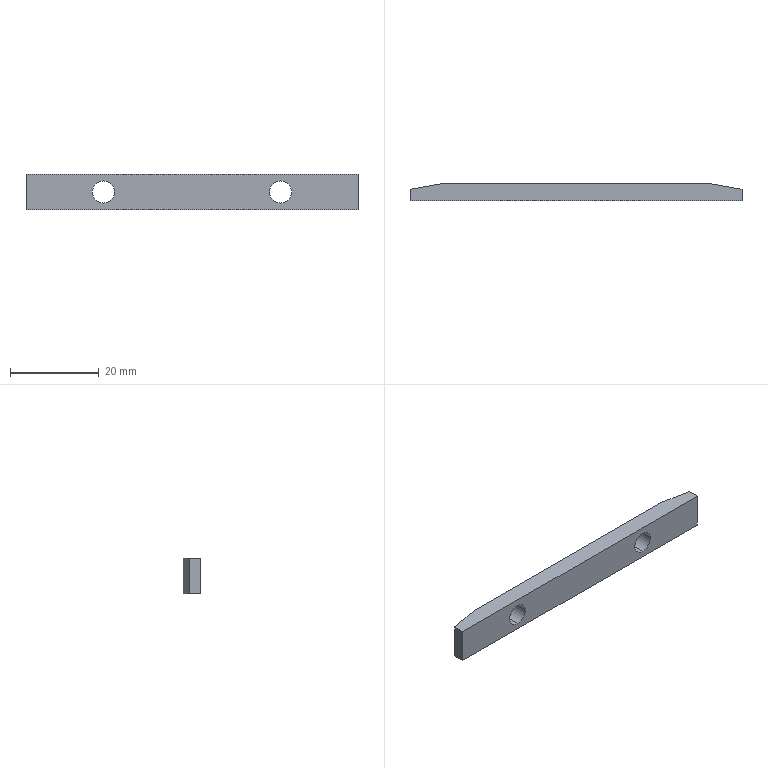Part | SolidWorks | features Chamfer 5, ICE 4, HoleWzd 2, Extrusion 1, Fillet 1 | 1 solid | 12 faces | box 75 x 4 x 8 mm | volume 2157 mm3 | plane 8 | cylinder 4 | commonest cylinder face diameters 5 x4
STEP:
#1=CARTESIAN_POINT('',(20.,45.,-2.5));
#2=VERTEX_POINT('',#1);
#3=CARTESIAN_POINT('',(20.,45.,2.5));
#4=VERTEX_POINT('',#3);
#5=CARTESIAN_POINT('',(20.,45.,0.));
#6=DIRECTION('',(0.,1.,0.));
#7=DIRECTION('',(0.,0.,1.));
#8=AXIS2_PLACEMENT_3D('',#5,#6,#7);
#9=CIRCLE('',#8,2.5);
#10=EDGE_CURVE('',#2,#4,#9,.T.);
#11=ORIENTED_EDGE('',*,*,#10,.F.);
#12=CARTESIAN_POINT('',(20.,49.,-2.5));
#13=VERTEX_POINT('',#12);
#14=CARTESIAN_POINT('',(20.,32.5,-2.5));
#15=DIRECTION('',(0.,1.,0.));
#16=VECTOR('',#15,1000.);
#17=LINE('',#14,#16);
#18=EDGE_CURVE('',#2,#13,#17,.T.);
#19=ORIENTED_EDGE('',*,*,#18,.T.);
#20=CARTESIAN_POINT('',(20.,49.,2.5));
#21=VERTEX_POINT('',#20);
#22=CARTESIAN_POINT('',(20.,49.,0.));
#23=DIRECTION('',(0.,1.,0.));
#24=DIRECTION('',(0.,0.,1.));
#25=AXIS2_PLACEMENT_3D('',#22,#23,#24);
#26=CIRCLE('',#25,2.5);
#27=EDGE_CURVE('',#13,#21,#26,.T.);
#28=ORIENTED_EDGE('',*,*,#27,.T.);
#29=CARTESIAN_POINT('',(20.,32.5,2.5));
#30=DIRECTION('',(0.,1.,0.));
#31=VECTOR('',#30,1000.);
#32=LINE('',#29,#31);
#33=EDGE_CURVE('',#4,#21,#32,.T.);
#34=ORIENTED_EDGE('',*,*,#33,.F.);
#35=EDGE_LOOP('',(#11,#19,#28,#34));
#36=FACE_OUTER_BOUND('',#35,.T.);
#37=CARTESIAN_POINT('',(20.,32.5,0.));
#38=DIRECTION('',(0.,1.,0.));
#39=DIRECTION('',(0.,0.,1.));
#40=AXIS2_PLACEMENT_3D('',#37,#38,#39);
#41=CYLINDRICAL_SURFACE('',#40,2.5);
#42=ADVANCED_FACE('',(#36),#41,.F.);
#43=CARTESIAN_POINT('',(-20.,45.,-2.5));
#44=VERTEX_POINT('',#43);
#45=CARTESIAN_POINT('',(-20.,45.,2.5));
#46=VERTEX_POINT('',#45);
#47=CARTESIAN_POINT('',(-20.,45.,0.));
#48=DIRECTION('',(0.,1.,0.));
#49=DIRECTION('',(0.,0.,1.));
#50=AXIS2_PLACEMENT_3D('',#47,#48,#49);
#51=CIRCLE('',#50,2.5);
#52=EDGE_CURVE('',#44,#46,#51,.T.);
#53=ORIENTED_EDGE('',*,*,#52,.F.);
#54=CARTESIAN_POINT('',(-20.,49.,-2.5));
#55=VERTEX_POINT('',#54);
#56=CARTESIAN_POINT('',(-20.,32.5,-2.5));
#57=DIRECTION('',(0.,1.,0.));
#58=VECTOR('',#57,1000.);
#59=LINE('',#56,#58);
#60=EDGE_CURVE('',#44,#55,#59,.T.);
#61=ORIENTED_EDGE('',*,*,#60,.T.);
#62=CARTESIAN_POINT('',(-20.,49.,2.5));
#63=VERTEX_POINT('',#62);
#64=CARTESIAN_POINT('',(-20.,49.,0.));
#65=DIRECTION('',(0.,1.,0.));
#66=DIRECTION('',(0.,0.,1.));
#67=AXIS2_PLACEMENT_3D('',#64,#65,#66);
#68=CIRCLE('',#67,2.5);
#69=EDGE_CURVE('',#55,#63,#68,.T.);
#70=ORIENTED_EDGE('',*,*,#69,.T.);
#71=CARTESIAN_POINT('',(-20.,32.5,2.5));
#72=DIRECTION('',(0.,1.,0.));
#73=VECTOR('',#72,1000.);
#74=LINE('',#71,#73);
#75=EDGE_CURVE('',#46,#63,#74,.T.);
#76=ORIENTED_EDGE('',*,*,#75,.F.);
#77=EDGE_LOOP('',(#53,#61,#70,#76));
#78=FACE_OUTER_BOUND('',#77,.T.);
#79=CARTESIAN_POINT('',(-20.,32.5,0.));
#80=DIRECTION('',(0.,1.,0.));
#81=DIRECTION('',(0.,0.,1.));
#82=AXIS2_PLACEMENT_3D('',#79,#80,#81);
#83=CYLINDRICAL_SURFACE('',#82,2.5);
#84=ADVANCED_FACE('',(#78),#83,.F.);
#85=CARTESIAN_POINT('',(37.5,45.,4.));
#86=VERTEX_POINT('',#85);
#87=CARTESIAN_POINT('',(-37.5,45.,4.));
#88=VERTEX_POINT('',#87);
#89=CARTESIAN_POINT('',(-71.258,45.,4.));
#90=DIRECTION('',(-1.,0.,0.));
#91=VECTOR('',#90,1000.);
#92=LINE('',#89,#91);
#93=EDGE_CURVE('',#86,#88,#92,.T.);
#94=ORIENTED_EDGE('',*,*,#93,.F.);
#95=CARTESIAN_POINT('',(37.5,47.6,4.));
#96=VERTEX_POINT('',#95);
#97=CARTESIAN_POINT('',(37.5,49.,4.));
#98=DIRECTION('',(0.,1.,0.));
#99=VECTOR('',#98,1000.);
#100=LINE('',#97,#99);
#101=EDGE_CURVE('',#86,#96,#100,.T.);
#102=ORIENTED_EDGE('',*,*,#101,.T.);
#103=CARTESIAN_POINT('',(29.8,49.,4.));
#104=VERTEX_POINT('',#103);
#105=CARTESIAN_POINT('',(9.578,52.677,4.));
#106=DIRECTION('',(-0.9839,0.1789,0.));
#107=VECTOR('',#106,1000.);
#108=LINE('',#105,#107);
#109=EDGE_CURVE('',#96,#104,#108,.T.);
#110=ORIENTED_EDGE('',*,*,#109,.T.);
#111=CARTESIAN_POINT('',(-29.8,49.,4.));
#112=VERTEX_POINT('',#111);
#113=CARTESIAN_POINT('',(-37.5,49.,4.));
#114=DIRECTION('',(-1.,0.,0.));
#115=VECTOR('',#114,1000.);
#116=LINE('',#113,#115);
#117=EDGE_CURVE('',#104,#112,#116,.T.);
#118=ORIENTED_EDGE('',*,*,#117,.T.);
#119=CARTESIAN_POINT('',(-37.5,47.6,4.));
#120=VERTEX_POINT('',#119);
#121=CARTESIAN_POINT('',(-9.578,52.677,4.));
#122=DIRECTION('',(-0.9839,-0.1789,0.));
#123=VECTOR('',#122,1000.);
#124=LINE('',#121,#123);
#125=EDGE_CURVE('',#112,#120,#124,.T.);
#126=ORIENTED_EDGE('',*,*,#125,.T.);
#127=CARTESIAN_POINT('',(-37.5,49.,4.));
#128=DIRECTION('',(0.,-1.,0.));
#129=VECTOR('',#128,1000.);
#130=LINE('',#127,#129);
#131=EDGE_CURVE('',#120,#88,#130,.T.);
#132=ORIENTED_EDGE('',*,*,#131,.T.);
#133=EDGE_LOOP('',(#94,#102,#110,#118,#126,#132));
#134=FACE_OUTER_BOUND('',#133,.T.);
#135=CARTESIAN_POINT('',(0.,0.,4.));
#136=DIRECTION('',(0.,0.,1.));
#137=DIRECTION('',(1.,0.,0.));
#138=AXIS2_PLACEMENT_3D('',#135,#136,#137);
#139=PLANE('',#138);
#140=ADVANCED_FACE('',(#134),#139,.T.);
#141=CARTESIAN_POINT('',(37.5,45.,-4.));
#142=VERTEX_POINT('',#141);
#143=CARTESIAN_POINT('',(37.5,47.6,-4.));
#144=VERTEX_POINT('',#143);
#145=CARTESIAN_POINT('',(37.5,49.,-4.));
#146=DIRECTION('',(0.,1.,0.));
#147=VECTOR('',#146,1000.);
#148=LINE('',#145,#147);
#149=EDGE_CURVE('',#142,#144,#148,.T.);
#150=ORIENTED_EDGE('',*,*,#149,.F.);
#151=CARTESIAN_POINT('',(-37.5,45.,-4.));
#152=VERTEX_POINT('',#151);
#153=CARTESIAN_POINT('',(0.,45.,-4.));
#154=DIRECTION('',(-1.,0.,0.));
#155=VECTOR('',#154,1000.);
#156=LINE('',#153,#155);
#157=EDGE_CURVE('',#142,#152,#156,.T.);
#158=ORIENTED_EDGE('',*,*,#157,.T.);
#159=CARTESIAN_POINT('',(-37.5,47.6,-4.));
#160=VERTEX_POINT('',#159);
#161=CARTESIAN_POINT('',(-37.5,49.,-4.));
#162=DIRECTION('',(0.,-1.,0.));
#163=VECTOR('',#162,1000.);
#164=LINE('',#161,#163);
#165=EDGE_CURVE('',#160,#152,#164,.T.);
#166=ORIENTED_EDGE('',*,*,#165,.F.);
#167=CARTESIAN_POINT('',(-29.8,49.,-4.));
#168=VERTEX_POINT('',#167);
#169=CARTESIAN_POINT('',(-37.5,47.6,-4.));
#170=DIRECTION('',(0.9839,0.1789,0.));
#171=VECTOR('',#170,1000.);
#172=LINE('',#169,#171);
#173=EDGE_CURVE('',#160,#168,#172,.T.);
#174=ORIENTED_EDGE('',*,*,#173,.T.);
#175=CARTESIAN_POINT('',(29.8,49.,-4.));
#176=VERTEX_POINT('',#175);
#177=CARTESIAN_POINT('',(-37.5,49.,-4.));
#178=DIRECTION('',(-1.,0.,0.));
#179=VECTOR('',#178,1000.);
#180=LINE('',#177,#179);
#181=EDGE_CURVE('',#176,#168,#180,.T.);
#182=ORIENTED_EDGE('',*,*,#181,.F.);
#183=CARTESIAN_POINT('',(29.8,49.,-4.));
#184=DIRECTION('',(0.9839,-0.1789,0.));
#185=VECTOR('',#184,1000.);
#186=LINE('',#183,#185);
#187=EDGE_CURVE('',#176,#144,#186,.T.);
#188=ORIENTED_EDGE('',*,*,#187,.T.);
#189=EDGE_LOOP('',(#150,#158,#166,#174,#182,#188));
#190=FACE_OUTER_BOUND('',#189,.T.);
#191=CARTESIAN_POINT('',(0.,0.,-4.));
#192=DIRECTION('',(0.,0.,1.));
#193=DIRECTION('',(1.,0.,0.));
#194=AXIS2_PLACEMENT_3D('',#191,#192,#193);
#195=PLANE('',#194);
#196=ADVANCED_FACE('',(#190),#195,.F.);
#197=ORIENTED_EDGE('',*,*,#101,.F.);
#198=CARTESIAN_POINT('',(37.5,45.,4.));
#199=DIRECTION('',(0.,0.,-1.));
#200=VECTOR('',#199,1000.);
#201=LINE('',#198,#200);
#202=EDGE_CURVE('',#86,#142,#201,.T.);
#203=ORIENTED_EDGE('',*,*,#202,.T.);
#204=ORIENTED_EDGE('',*,*,#149,.T.);
#205=CARTESIAN_POINT('',(37.5,47.6,4.));
#206=DIRECTION('',(0.,0.,1.));
#207=VECTOR('',#206,1000.);
#208=LINE('',#205,#207);
#209=EDGE_CURVE('',#144,#96,#208,.T.);
#210=ORIENTED_EDGE('',*,*,#209,.T.);
#211=EDGE_LOOP('',(#197,#203,#204,#210));
#212=FACE_OUTER_BOUND('',#211,.T.);
#213=CARTESIAN_POINT('',(37.5,49.,4.));
#214=DIRECTION('',(-1.,0.,0.));
#215=DIRECTION('',(0.,0.,1.));
#216=AXIS2_PLACEMENT_3D('',#213,#214,#215);
#217=PLANE('',#216);
#218=ADVANCED_FACE('',(#212),#217,.F.);
#219=CARTESIAN_POINT('',(20.,49.,0.));
#220=DIRECTION('',(0.,1.,0.));
#221=DIRECTION('',(0.,0.,1.));
#222=AXIS2_PLACEMENT_3D('',#219,#220,#221);
#223=CIRCLE('',#222,2.5);
#224=EDGE_CURVE('',#21,#13,#223,.T.);
#225=ORIENTED_EDGE('',*,*,#224,.F.);
#226=ORIENTED_EDGE('',*,*,#27,.F.);
#227=EDGE_LOOP('',(#225,#226));
#228=FACE_BOUND('',#227,.T.);
#229=CARTESIAN_POINT('',(-20.,49.,0.));
#230=DIRECTION('',(0.,1.,0.));
#231=DIRECTION('',(0.,0.,1.));
#232=AXIS2_PLACEMENT_3D('',#229,#230,#231);
#233=CIRCLE('',#232,2.5);
#234=EDGE_CURVE('',#63,#55,#233,.T.);
#235=ORIENTED_EDGE('',*,*,#234,.F.);
#236=ORIENTED_EDGE('',*,*,#69,.F.);
#237=EDGE_LOOP('',(#235,#236));
#238=FACE_BOUND('',#237,.T.);
#239=ORIENTED_EDGE('',*,*,#117,.F.);
#240=CARTESIAN_POINT('',(29.8,49.,4.));
#241=DIRECTION('',(0.,0.,-1.));
#242=VECTOR('',#241,1000.);
#243=LINE('',#240,#242);
#244=EDGE_CURVE('',#104,#176,#243,.T.);
#245=ORIENTED_EDGE('',*,*,#244,.T.);
#246=ORIENTED_EDGE('',*,*,#181,.T.);
#247=CARTESIAN_POINT('',(-29.8,49.,4.));
#248=DIRECTION('',(0.,0.,1.));
#249=VECTOR('',#248,1000.);
#250=LINE('',#247,#249);
#251=EDGE_CURVE('',#168,#112,#250,.T.);
#252=ORIENTED_EDGE('',*,*,#251,.T.);
#253=EDGE_LOOP('',(#239,#245,#246,#252));
#254=FACE_OUTER_BOUND('',#253,.T.);
#255=CARTESIAN_POINT('',(-37.5,49.,4.));
#256=DIRECTION('',(0.,-1.,0.));
#257=DIRECTION('',(0.,0.,-1.));
#258=AXIS2_PLACEMENT_3D('',#255,#256,#257);
#259=PLANE('',#258);
#260=ADVANCED_FACE('',(#228,#238,#254),#259,.F.);
#261=ORIENTED_EDGE('',*,*,#165,.T.);
#262=CARTESIAN_POINT('',(-37.5,45.,4.));
#263=DIRECTION('',(0.,0.,1.));
#264=VECTOR('',#263,1000.);
#265=LINE('',#262,#264);
#266=EDGE_CURVE('',#152,#88,#265,.T.);
#267=ORIENTED_EDGE('',*,*,#266,.T.);
#268=ORIENTED_EDGE('',*,*,#131,.F.);
#269=CARTESIAN_POINT('',(-37.5,47.6,4.));
#270=DIRECTION('',(0.,0.,-1.));
#271=VECTOR('',#270,1000.);
#272=LINE('',#269,#271);
#273=EDGE_CURVE('',#120,#160,#272,.T.);
#274=ORIENTED_EDGE('',*,*,#273,.T.);
#275=EDGE_LOOP('',(#261,#267,#268,#274));
#276=FACE_OUTER_BOUND('',#275,.T.);
#277=CARTESIAN_POINT('',(-37.5,49.,4.));
#278=DIRECTION('',(1.,0.,0.));
#279=DIRECTION('',(0.,1.,0.));
#280=AXIS2_PLACEMENT_3D('',#277,#278,#279);
#281=PLANE('',#280);
#282=ADVANCED_FACE('',(#276),#281,.F.);
#283=ORIENTED_EDGE('',*,*,#125,.F.);
#284=ORIENTED_EDGE('',*,*,#251,.F.);
#285=ORIENTED_EDGE('',*,*,#173,.F.);
#286=ORIENTED_EDGE('',*,*,#273,.F.);
#287=EDGE_LOOP('',(#283,#284,#285,#286));
#288=FACE_OUTER_BOUND('',#287,.T.);
#289=CARTESIAN_POINT('',(-37.5,47.6,4.));
#290=DIRECTION('',(0.1789,-0.9839,0.));
#291=DIRECTION('',(0.,0.,-1.));
#292=AXIS2_PLACEMENT_3D('',#289,#290,#291);
#293=PLANE('',#292);
#294=ADVANCED_FACE('',(#288),#293,.F.);
#295=ORIENTED_EDGE('',*,*,#109,.F.);
#296=ORIENTED_EDGE('',*,*,#209,.F.);
#297=ORIENTED_EDGE('',*,*,#187,.F.);
#298=ORIENTED_EDGE('',*,*,#244,.F.);
#299=EDGE_LOOP('',(#295,#296,#297,#298));
#300=FACE_OUTER_BOUND('',#299,.T.);
#301=CARTESIAN_POINT('',(29.8,49.,4.));
#302=DIRECTION('',(-0.1789,-0.9839,0.));
#303=DIRECTION('',(0.,0.,-1.));
#304=AXIS2_PLACEMENT_3D('',#301,#302,#303);
#305=PLANE('',#304);
#306=ADVANCED_FACE('',(#300),#305,.F.);
#307=CARTESIAN_POINT('',(20.,45.,0.));
#308=DIRECTION('',(0.,1.,0.));
#309=DIRECTION('',(0.,0.,1.));
#310=AXIS2_PLACEMENT_3D('',#307,#308,#309);
#311=CIRCLE('',#310,2.5);
#312=EDGE_CURVE('',#4,#2,#311,.T.);
#313=ORIENTED_EDGE('',*,*,#312,.T.);
#314=ORIENTED_EDGE('',*,*,#10,.T.);
#315=EDGE_LOOP('',(#313,#314));
#316=FACE_BOUND('',#315,.T.);
#317=CARTESIAN_POINT('',(-20.,45.,0.));
#318=DIRECTION('',(0.,1.,0.));
#319=DIRECTION('',(0.,0.,1.));
#320=AXIS2_PLACEMENT_3D('',#317,#318,#319);
#321=CIRCLE('',#320,2.5);
#322=EDGE_CURVE('',#46,#44,#321,.T.);
#323=ORIENTED_EDGE('',*,*,#322,.T.);
#324=ORIENTED_EDGE('',*,*,#52,.T.);
#325=EDGE_LOOP('',(#323,#324));
#326=FACE_BOUND('',#325,.T.);
#327=ORIENTED_EDGE('',*,*,#93,.T.);
#328=ORIENTED_EDGE('',*,*,#266,.F.);
#329=ORIENTED_EDGE('',*,*,#157,.F.);
#330=ORIENTED_EDGE('',*,*,#202,.F.);
#331=EDGE_LOOP('',(#327,#328,#329,#330));
#332=FACE_OUTER_BOUND('',#331,.T.);
#333=CARTESIAN_POINT('',(-71.258,45.,-39.));
#334=DIRECTION('',(0.,1.,0.));
#335=DIRECTION('',(0.,0.,1.));
#336=AXIS2_PLACEMENT_3D('',#333,#334,#335);
#337=PLANE('',#336);
#338=ADVANCED_FACE('',(#316,#326,#332),#337,.F.);
#339=ORIENTED_EDGE('',*,*,#60,.F.);
#340=ORIENTED_EDGE('',*,*,#322,.F.);
#341=ORIENTED_EDGE('',*,*,#75,.T.);
#342=ORIENTED_EDGE('',*,*,#234,.T.);
#343=EDGE_LOOP('',(#339,#340,#341,#342));
#344=FACE_OUTER_BOUND('',#343,.T.);
#345=CARTESIAN_POINT('',(-20.,32.5,0.));
#346=DIRECTION('',(0.,1.,0.));
#347=DIRECTION('',(0.,0.,1.));
#348=AXIS2_PLACEMENT_3D('',#345,#346,#347);
#349=CYLINDRICAL_SURFACE('',#348,2.5);
#350=ADVANCED_FACE('',(#344),#349,.F.);
#351=ORIENTED_EDGE('',*,*,#18,.F.);
#352=ORIENTED_EDGE('',*,*,#312,.F.);
#353=ORIENTED_EDGE('',*,*,#33,.T.);
#354=ORIENTED_EDGE('',*,*,#224,.T.);
#355=EDGE_LOOP('',(#351,#352,#353,#354));
#356=FACE_OUTER_BOUND('',#355,.T.);
#357=CARTESIAN_POINT('',(20.,32.5,0.));
#358=DIRECTION('',(0.,1.,0.));
#359=DIRECTION('',(0.,0.,1.));
#360=AXIS2_PLACEMENT_3D('',#357,#358,#359);
#361=CYLINDRICAL_SURFACE('',#360,2.5);
#362=ADVANCED_FACE('',(#356),#361,.F.);
#363=CLOSED_SHELL('',(#42,#84,#140,#196,#218,#260,#282,#294,#306,#338,#350,#362));
#364=MANIFOLD_SOLID_BREP('',#363);
#365=CARTESIAN_POINT('',(0.,0.,0.));
#366=DIRECTION('',(0.,0.,1.));
#367=DIRECTION('',(1.,0.,0.));
#368=AXIS2_PLACEMENT_3D('',#365,#366,#367);
#369=(LENGTH_UNIT()NAMED_UNIT(*)SI_UNIT(.MILLI.,.METRE.));
#370=UNCERTAINTY_MEASURE_WITH_UNIT(LENGTH_MEASURE(0.00001),#369,'','');
#371=(NAMED_UNIT(*)PLANE_ANGLE_UNIT()SI_UNIT($,.RADIAN.));
#372=(NAMED_UNIT(*)SI_UNIT($,.STERADIAN.)SOLID_ANGLE_UNIT());
#373=(GEOMETRIC_REPRESENTATION_CONTEXT(3)GLOBAL_UNCERTAINTY_ASSIGNED_CONTEXT((#370))GLOBAL_UNIT_ASSIGNED_CONTEXT((#369,#371,#372))REPRESENTATION_CONTEXT('',''));
#374=ADVANCED_BREP_SHAPE_REPRESENTATION('',(#364,#368),#373);